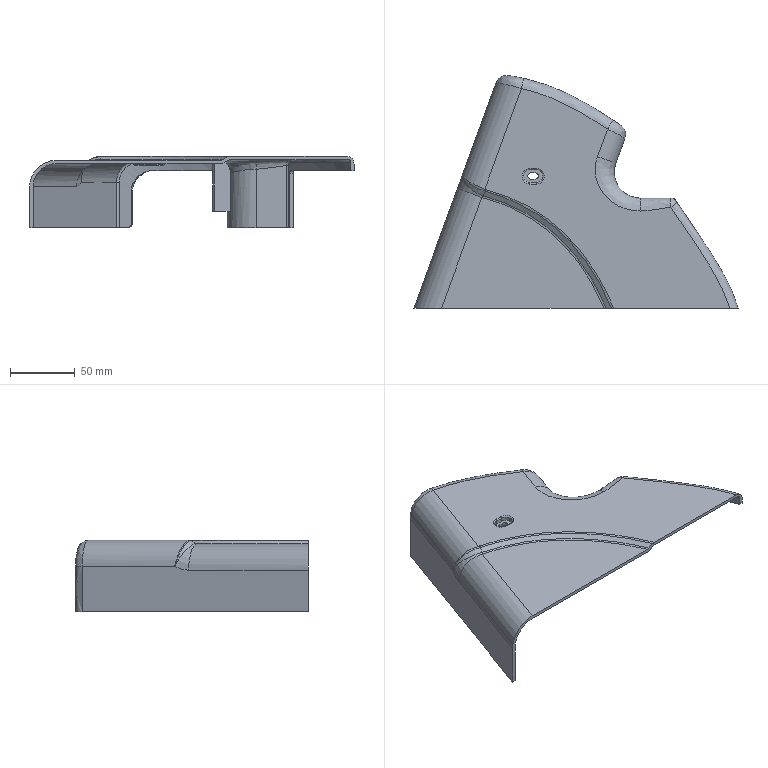Part | STEP file | LZHT-L1 | 1 solid | 102 faces | box 250 x 180.091 x 55 mm | volume 105552 mm3 | spline 40 | plane 30 | cylinder 26 | torus 6 | commonest cylinder face diameters 2 x6 4 x4 40 x3 5 x2 6 x2 10 x2